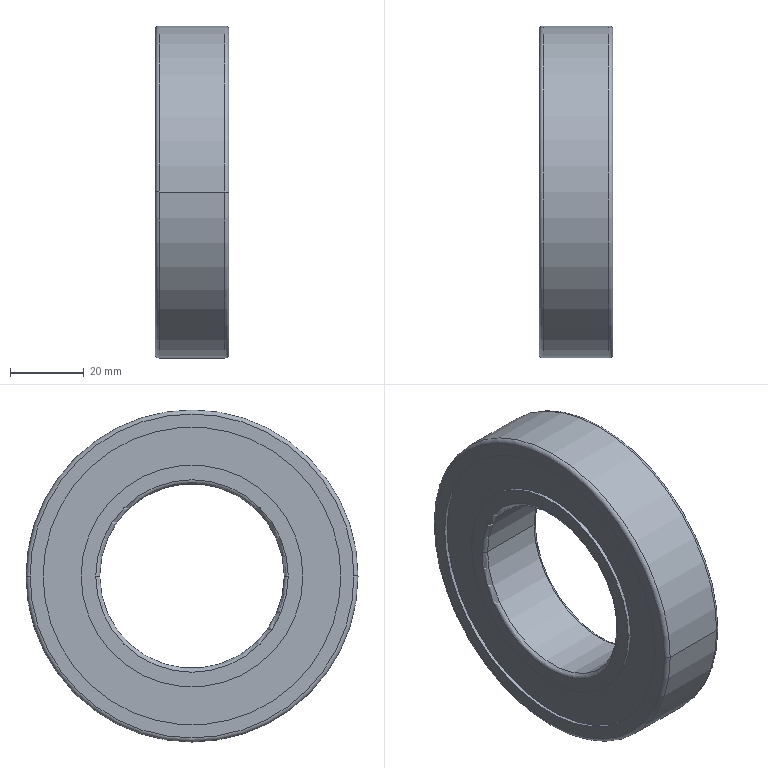Part | SolidWorks | features Fillet 2, Revolution 1 | 1 solid | 26 faces | box 20 x 90 x 90 mm | volume 83545 mm3 | cylinder 12 | torus 8 | plane 6 | commonest cylinder face diameters 60.1 x4 80.7 x4 50 x2 90 x2
STEP:
#1=CARTESIAN_POINT('',(1.1,-25.,0.));
#2=VERTEX_POINT('',#1);
#3=CARTESIAN_POINT('',(1.1,25.,0.));
#4=VERTEX_POINT('',#3);
#5=CARTESIAN_POINT('',(1.1,0.,0.));
#6=DIRECTION('',(-1.,0.,0.));
#7=DIRECTION('',(0.,1.,0.));
#8=AXIS2_PLACEMENT_3D('',#5,#6,#7);
#9=CIRCLE('',#8,25.);
#10=EDGE_CURVE('',#2,#4,#9,.T.);
#11=ORIENTED_EDGE('',*,*,#10,.F.);
#12=CARTESIAN_POINT('',(0.,-26.1,0.));
#13=VERTEX_POINT('',#12);
#14=CARTESIAN_POINT('',(1.1,-26.1,0.));
#15=DIRECTION('',(0.,0.,1.));
#16=DIRECTION('',(0.,-1.,0.));
#17=AXIS2_PLACEMENT_3D('',#14,#15,#16);
#18=CIRCLE('',#17,1.1);
#19=EDGE_CURVE('',#2,#13,#18,.T.);
#20=ORIENTED_EDGE('',*,*,#19,.T.);
#21=CARTESIAN_POINT('',(0.,26.1,0.));
#22=VERTEX_POINT('',#21);
#23=CARTESIAN_POINT('',(0.,0.,0.));
#24=DIRECTION('',(1.,0.,0.));
#25=DIRECTION('',(0.,1.,0.));
#26=AXIS2_PLACEMENT_3D('',#23,#24,#25);
#27=CIRCLE('',#26,26.1);
#28=EDGE_CURVE('',#22,#13,#27,.T.);
#29=ORIENTED_EDGE('',*,*,#28,.F.);
#30=CARTESIAN_POINT('',(1.1,26.1,0.));
#31=DIRECTION('',(0.,0.,-1.));
#32=DIRECTION('',(-1.,0.,0.));
#33=AXIS2_PLACEMENT_3D('',#30,#31,#32);
#34=CIRCLE('',#33,1.1);
#35=EDGE_CURVE('',#4,#22,#34,.T.);
#36=ORIENTED_EDGE('',*,*,#35,.F.);
#37=EDGE_LOOP('',(#11,#20,#29,#36));
#38=FACE_OUTER_BOUND('',#37,.T.);
#39=CARTESIAN_POINT('',(1.1,0.,0.));
#40=DIRECTION('',(1.,0.,0.));
#41=DIRECTION('',(0.,1.,0.));
#42=AXIS2_PLACEMENT_3D('',#39,#40,#41);
#43=TOROIDAL_SURFACE('',#42,26.1,1.1);
#44=ADVANCED_FACE('',(#38),#43,.T.);
#45=CARTESIAN_POINT('',(18.9,25.,0.));
#46=VERTEX_POINT('',#45);
#47=CARTESIAN_POINT('',(18.9,-25.,0.));
#48=VERTEX_POINT('',#47);
#49=CARTESIAN_POINT('',(18.9,0.,0.));
#50=DIRECTION('',(1.,0.,0.));
#51=DIRECTION('',(0.,-1.,0.));
#52=AXIS2_PLACEMENT_3D('',#49,#50,#51);
#53=CIRCLE('',#52,25.);
#54=EDGE_CURVE('',#46,#48,#53,.T.);
#55=ORIENTED_EDGE('',*,*,#54,.F.);
#56=CARTESIAN_POINT('',(20.,26.1,0.));
#57=VERTEX_POINT('',#56);
#58=CARTESIAN_POINT('',(18.9,26.1,0.));
#59=DIRECTION('',(0.,0.,1.));
#60=DIRECTION('',(0.,-1.,0.));
#61=AXIS2_PLACEMENT_3D('',#58,#59,#60);
#62=CIRCLE('',#61,1.1);
#63=EDGE_CURVE('',#46,#57,#62,.T.);
#64=ORIENTED_EDGE('',*,*,#63,.T.);
#65=CARTESIAN_POINT('',(20.,-26.1,0.));
#66=VERTEX_POINT('',#65);
#67=CARTESIAN_POINT('',(20.,0.,0.));
#68=DIRECTION('',(-1.,0.,0.));
#69=DIRECTION('',(0.,-1.,0.));
#70=AXIS2_PLACEMENT_3D('',#67,#68,#69);
#71=CIRCLE('',#70,26.1);
#72=EDGE_CURVE('',#66,#57,#71,.T.);
#73=ORIENTED_EDGE('',*,*,#72,.F.);
#74=CARTESIAN_POINT('',(18.9,-26.1,0.));
#75=DIRECTION('',(0.,0.,-1.));
#76=DIRECTION('',(-1.,0.,0.));
#77=AXIS2_PLACEMENT_3D('',#74,#75,#76);
#78=CIRCLE('',#77,1.1);
#79=EDGE_CURVE('',#48,#66,#78,.T.);
#80=ORIENTED_EDGE('',*,*,#79,.F.);
#81=EDGE_LOOP('',(#55,#64,#73,#80));
#82=FACE_OUTER_BOUND('',#81,.T.);
#83=CARTESIAN_POINT('',(18.9,0.,0.));
#84=DIRECTION('',(-1.,0.,0.));
#85=DIRECTION('',(0.,-1.,0.));
#86=AXIS2_PLACEMENT_3D('',#83,#84,#85);
#87=TOROIDAL_SURFACE('',#86,26.1,1.1);
#88=ADVANCED_FACE('',(#82),#87,.T.);
#89=CARTESIAN_POINT('',(0.,-43.9,0.));
#90=VERTEX_POINT('',#89);
#91=CARTESIAN_POINT('',(0.,43.9,0.));
#92=VERTEX_POINT('',#91);
#93=CARTESIAN_POINT('',(0.,0.,0.));
#94=DIRECTION('',(-1.,0.,0.));
#95=DIRECTION('',(0.,1.,0.));
#96=AXIS2_PLACEMENT_3D('',#93,#94,#95);
#97=CIRCLE('',#96,43.9);
#98=EDGE_CURVE('',#90,#92,#97,.T.);
#99=ORIENTED_EDGE('',*,*,#98,.F.);
#100=CARTESIAN_POINT('',(1.1,-45.,0.));
#101=VERTEX_POINT('',#100);
#102=CARTESIAN_POINT('',(1.1,-43.9,0.));
#103=DIRECTION('',(0.,0.,1.));
#104=DIRECTION('',(0.,-1.,0.));
#105=AXIS2_PLACEMENT_3D('',#102,#103,#104);
#106=CIRCLE('',#105,1.1);
#107=EDGE_CURVE('',#90,#101,#106,.T.);
#108=ORIENTED_EDGE('',*,*,#107,.T.);
#109=CARTESIAN_POINT('',(1.1,45.,0.));
#110=VERTEX_POINT('',#109);
#111=CARTESIAN_POINT('',(1.1,0.,0.));
#112=DIRECTION('',(1.,0.,0.));
#113=DIRECTION('',(0.,1.,0.));
#114=AXIS2_PLACEMENT_3D('',#111,#112,#113);
#115=CIRCLE('',#114,45.);
#116=EDGE_CURVE('',#110,#101,#115,.T.);
#117=ORIENTED_EDGE('',*,*,#116,.F.);
#118=CARTESIAN_POINT('',(1.1,43.9,0.));
#119=DIRECTION('',(0.,0.,-1.));
#120=DIRECTION('',(-1.,0.,0.));
#121=AXIS2_PLACEMENT_3D('',#118,#119,#120);
#122=CIRCLE('',#121,1.1);
#123=EDGE_CURVE('',#92,#110,#122,.T.);
#124=ORIENTED_EDGE('',*,*,#123,.F.);
#125=EDGE_LOOP('',(#99,#108,#117,#124));
#126=FACE_OUTER_BOUND('',#125,.T.);
#127=CARTESIAN_POINT('',(1.1,0.,0.));
#128=DIRECTION('',(1.,0.,0.));
#129=DIRECTION('',(0.,1.,0.));
#130=AXIS2_PLACEMENT_3D('',#127,#128,#129);
#131=TOROIDAL_SURFACE('',#130,43.9,1.1);
#132=ADVANCED_FACE('',(#126),#131,.T.);
#133=CARTESIAN_POINT('',(20.,43.9,0.));
#134=VERTEX_POINT('',#133);
#135=CARTESIAN_POINT('',(20.,-43.9,0.));
#136=VERTEX_POINT('',#135);
#137=CARTESIAN_POINT('',(20.,0.,0.));
#138=DIRECTION('',(1.,0.,0.));
#139=DIRECTION('',(0.,-1.,0.));
#140=AXIS2_PLACEMENT_3D('',#137,#138,#139);
#141=CIRCLE('',#140,43.9);
#142=EDGE_CURVE('',#134,#136,#141,.T.);
#143=ORIENTED_EDGE('',*,*,#142,.F.);
#144=CARTESIAN_POINT('',(18.9,45.,0.));
#145=VERTEX_POINT('',#144);
#146=CARTESIAN_POINT('',(18.9,43.9,0.));
#147=DIRECTION('',(0.,0.,1.));
#148=DIRECTION('',(0.,-1.,0.));
#149=AXIS2_PLACEMENT_3D('',#146,#147,#148);
#150=CIRCLE('',#149,1.1);
#151=EDGE_CURVE('',#134,#145,#150,.T.);
#152=ORIENTED_EDGE('',*,*,#151,.T.);
#153=CARTESIAN_POINT('',(18.9,-45.,0.));
#154=VERTEX_POINT('',#153);
#155=CARTESIAN_POINT('',(18.9,0.,0.));
#156=DIRECTION('',(-1.,0.,0.));
#157=DIRECTION('',(0.,-1.,0.));
#158=AXIS2_PLACEMENT_3D('',#155,#156,#157);
#159=CIRCLE('',#158,45.);
#160=EDGE_CURVE('',#154,#145,#159,.T.);
#161=ORIENTED_EDGE('',*,*,#160,.F.);
#162=CARTESIAN_POINT('',(18.9,-43.9,0.));
#163=DIRECTION('',(0.,0.,-1.));
#164=DIRECTION('',(-1.,0.,0.));
#165=AXIS2_PLACEMENT_3D('',#162,#163,#164);
#166=CIRCLE('',#165,1.1);
#167=EDGE_CURVE('',#136,#154,#166,.T.);
#168=ORIENTED_EDGE('',*,*,#167,.F.);
#169=EDGE_LOOP('',(#143,#152,#161,#168));
#170=FACE_OUTER_BOUND('',#169,.T.);
#171=CARTESIAN_POINT('',(18.9,0.,0.));
#172=DIRECTION('',(-1.,0.,0.));
#173=DIRECTION('',(0.,-1.,0.));
#174=AXIS2_PLACEMENT_3D('',#171,#172,#173);
#175=TOROIDAL_SURFACE('',#174,43.9,1.1);
#176=ADVANCED_FACE('',(#170),#175,.T.);
#177=ORIENTED_EDGE('',*,*,#160,.T.);
#178=CARTESIAN_POINT('',(0.,45.,0.));
#179=DIRECTION('',(-1.,0.,0.));
#180=VECTOR('',#179,1000.);
#181=LINE('',#178,#180);
#182=EDGE_CURVE('',#145,#110,#181,.T.);
#183=ORIENTED_EDGE('',*,*,#182,.T.);
#184=ORIENTED_EDGE('',*,*,#116,.T.);
#185=CARTESIAN_POINT('',(0.,-45.,0.));
#186=DIRECTION('',(-1.,0.,0.));
#187=VECTOR('',#186,1000.);
#188=LINE('',#185,#187);
#189=EDGE_CURVE('',#154,#101,#188,.T.);
#190=ORIENTED_EDGE('',*,*,#189,.F.);
#191=EDGE_LOOP('',(#177,#183,#184,#190));
#192=FACE_OUTER_BOUND('',#191,.T.);
#193=CARTESIAN_POINT('',(0.,0.,0.));
#194=DIRECTION('',(-1.,0.,0.));
#195=DIRECTION('',(0.,-1.,0.));
#196=AXIS2_PLACEMENT_3D('',#193,#194,#195);
#197=CYLINDRICAL_SURFACE('',#196,45.);
#198=ADVANCED_FACE('',(#192),#197,.T.);
#199=CARTESIAN_POINT('',(20.,40.35,0.));
#200=VERTEX_POINT('',#199);
#201=CARTESIAN_POINT('',(20.,-40.35,0.));
#202=VERTEX_POINT('',#201);
#203=CARTESIAN_POINT('',(20.,0.,0.));
#204=DIRECTION('',(-1.,0.,0.));
#205=DIRECTION('',(0.,-1.,0.));
#206=AXIS2_PLACEMENT_3D('',#203,#204,#205);
#207=CIRCLE('',#206,40.35);
#208=EDGE_CURVE('',#200,#202,#207,.T.);
#209=ORIENTED_EDGE('',*,*,#208,.F.);
#210=CARTESIAN_POINT('',(19.08,40.35,0.));
#211=VERTEX_POINT('',#210);
#212=CARTESIAN_POINT('',(0.,40.35,0.));
#213=DIRECTION('',(-1.,0.,0.));
#214=VECTOR('',#213,1000.);
#215=LINE('',#212,#214);
#216=EDGE_CURVE('',#200,#211,#215,.T.);
#217=ORIENTED_EDGE('',*,*,#216,.T.);
#218=CARTESIAN_POINT('',(19.08,-40.35,0.));
#219=VERTEX_POINT('',#218);
#220=CARTESIAN_POINT('',(19.08,0.,0.));
#221=DIRECTION('',(-1.,0.,0.));
#222=DIRECTION('',(0.,-1.,0.));
#223=AXIS2_PLACEMENT_3D('',#220,#221,#222);
#224=CIRCLE('',#223,40.35);
#225=EDGE_CURVE('',#211,#219,#224,.T.);
#226=ORIENTED_EDGE('',*,*,#225,.T.);
#227=CARTESIAN_POINT('',(0.,-40.35,0.));
#228=DIRECTION('',(-1.,0.,0.));
#229=VECTOR('',#228,1000.);
#230=LINE('',#227,#229);
#231=EDGE_CURVE('',#202,#219,#230,.T.);
#232=ORIENTED_EDGE('',*,*,#231,.F.);
#233=EDGE_LOOP('',(#209,#217,#226,#232));
#234=FACE_OUTER_BOUND('',#233,.T.);
#235=CARTESIAN_POINT('',(0.,0.,0.));
#236=DIRECTION('',(-1.,0.,0.));
#237=DIRECTION('',(0.,-1.,0.));
#238=AXIS2_PLACEMENT_3D('',#235,#236,#237);
#239=CYLINDRICAL_SURFACE('',#238,40.35);
#240=ADVANCED_FACE('',(#234),#239,.F.);
#241=CARTESIAN_POINT('',(20.,-30.05,0.));
#242=VERTEX_POINT('',#241);
#243=CARTESIAN_POINT('',(20.,30.05,0.));
#244=VERTEX_POINT('',#243);
#245=CARTESIAN_POINT('',(20.,0.,0.));
#246=DIRECTION('',(-1.,0.,0.));
#247=DIRECTION('',(0.,-1.,0.));
#248=AXIS2_PLACEMENT_3D('',#245,#246,#247);
#249=CIRCLE('',#248,30.05);
#250=EDGE_CURVE('',#242,#244,#249,.T.);
#251=ORIENTED_EDGE('',*,*,#250,.T.);
#252=CARTESIAN_POINT('',(19.08,30.05,0.));
#253=VERTEX_POINT('',#252);
#254=CARTESIAN_POINT('',(0.,30.05,0.));
#255=DIRECTION('',(-1.,0.,0.));
#256=VECTOR('',#255,1000.);
#257=LINE('',#254,#256);
#258=EDGE_CURVE('',#244,#253,#257,.T.);
#259=ORIENTED_EDGE('',*,*,#258,.T.);
#260=CARTESIAN_POINT('',(19.08,-30.05,0.));
#261=VERTEX_POINT('',#260);
#262=CARTESIAN_POINT('',(19.08,0.,0.));
#263=DIRECTION('',(-1.,0.,0.));
#264=DIRECTION('',(0.,-1.,0.));
#265=AXIS2_PLACEMENT_3D('',#262,#263,#264);
#266=CIRCLE('',#265,30.05);
#267=EDGE_CURVE('',#261,#253,#266,.T.);
#268=ORIENTED_EDGE('',*,*,#267,.F.);
#269=CARTESIAN_POINT('',(0.,-30.05,0.));
#270=DIRECTION('',(-1.,0.,0.));
#271=VECTOR('',#270,1000.);
#272=LINE('',#269,#271);
#273=EDGE_CURVE('',#242,#261,#272,.T.);
#274=ORIENTED_EDGE('',*,*,#273,.F.);
#275=EDGE_LOOP('',(#251,#259,#268,#274));
#276=FACE_OUTER_BOUND('',#275,.T.);
#277=CARTESIAN_POINT('',(0.,0.,0.));
#278=DIRECTION('',(-1.,0.,0.));
#279=DIRECTION('',(0.,-1.,0.));
#280=AXIS2_PLACEMENT_3D('',#277,#278,#279);
#281=CYLINDRICAL_SURFACE('',#280,30.05);
#282=ADVANCED_FACE('',(#276),#281,.T.);
#283=CARTESIAN_POINT('',(18.9,0.,0.));
#284=DIRECTION('',(1.,0.,0.));
#285=DIRECTION('',(0.,-1.,0.));
#286=AXIS2_PLACEMENT_3D('',#283,#284,#285);
#287=CIRCLE('',#286,25.);
#288=EDGE_CURVE('',#48,#46,#287,.T.);
#289=ORIENTED_EDGE('',*,*,#288,.T.);
#290=CARTESIAN_POINT('',(0.,25.,0.));
#291=DIRECTION('',(-1.,0.,0.));
#292=VECTOR('',#291,1000.);
#293=LINE('',#290,#292);
#294=EDGE_CURVE('',#46,#4,#293,.T.);
#295=ORIENTED_EDGE('',*,*,#294,.T.);
#296=CARTESIAN_POINT('',(1.1,0.,0.));
#297=DIRECTION('',(-1.,0.,0.));
#298=DIRECTION('',(0.,1.,0.));
#299=AXIS2_PLACEMENT_3D('',#296,#297,#298);
#300=CIRCLE('',#299,25.);
#301=EDGE_CURVE('',#4,#2,#300,.T.);
#302=ORIENTED_EDGE('',*,*,#301,.T.);
#303=CARTESIAN_POINT('',(0.,-25.,0.));
#304=DIRECTION('',(-1.,0.,0.));
#305=VECTOR('',#304,1000.);
#306=LINE('',#303,#305);
#307=EDGE_CURVE('',#48,#2,#306,.T.);
#308=ORIENTED_EDGE('',*,*,#307,.F.);
#309=EDGE_LOOP('',(#289,#295,#302,#308));
#310=FACE_OUTER_BOUND('',#309,.T.);
#311=CARTESIAN_POINT('',(0.,0.,0.));
#312=DIRECTION('',(-1.,0.,0.));
#313=DIRECTION('',(0.,-1.,0.));
#314=AXIS2_PLACEMENT_3D('',#311,#312,#313);
#315=CYLINDRICAL_SURFACE('',#314,25.);
#316=ADVANCED_FACE('',(#310),#315,.F.);
#317=CARTESIAN_POINT('',(0.92,-30.05,0.));
#318=VERTEX_POINT('',#317);
#319=CARTESIAN_POINT('',(0.92,30.05,0.));
#320=VERTEX_POINT('',#319);
#321=CARTESIAN_POINT('',(0.92,0.,0.));
#322=DIRECTION('',(-1.,0.,0.));
#323=DIRECTION('',(0.,-1.,0.));
#324=AXIS2_PLACEMENT_3D('',#321,#322,#323);
#325=CIRCLE('',#324,30.05);
#326=EDGE_CURVE('',#318,#320,#325,.T.);
#327=ORIENTED_EDGE('',*,*,#326,.T.);
#328=CARTESIAN_POINT('',(0.,30.05,0.));
#329=VERTEX_POINT('',#328);
#330=CARTESIAN_POINT('',(0.,30.05,0.));
#331=DIRECTION('',(-1.,0.,0.));
#332=VECTOR('',#331,1000.);
#333=LINE('',#330,#332);
#334=EDGE_CURVE('',#320,#329,#333,.T.);
#335=ORIENTED_EDGE('',*,*,#334,.T.);
#336=CARTESIAN_POINT('',(0.,-30.05,0.));
#337=VERTEX_POINT('',#336);
#338=CARTESIAN_POINT('',(0.,0.,0.));
#339=DIRECTION('',(-1.,0.,0.));
#340=DIRECTION('',(0.,-1.,0.));
#341=AXIS2_PLACEMENT_3D('',#338,#339,#340);
#342=CIRCLE('',#341,30.05);
#343=EDGE_CURVE('',#337,#329,#342,.T.);
#344=ORIENTED_EDGE('',*,*,#343,.F.);
#345=CARTESIAN_POINT('',(0.,-30.05,0.));
#346=DIRECTION('',(-1.,0.,0.));
#347=VECTOR('',#346,1000.);
#348=LINE('',#345,#347);
#349=EDGE_CURVE('',#318,#337,#348,.T.);
#350=ORIENTED_EDGE('',*,*,#349,.F.);
#351=EDGE_LOOP('',(#327,#335,#344,#350));
#352=FACE_OUTER_BOUND('',#351,.T.);
#353=CARTESIAN_POINT('',(0.,0.,0.));
#354=DIRECTION('',(-1.,0.,0.));
#355=DIRECTION('',(0.,-1.,0.));
#356=AXIS2_PLACEMENT_3D('',#353,#354,#355);
#357=CYLINDRICAL_SURFACE('',#356,30.05);
#358=ADVANCED_FACE('',(#352),#357,.T.);
#359=CARTESIAN_POINT('',(0.92,40.35,0.));
#360=VERTEX_POINT('',#359);
#361=CARTESIAN_POINT('',(0.92,-40.35,0.));
#362=VERTEX_POINT('',#361);
#363=CARTESIAN_POINT('',(0.92,0.,0.));
#364=DIRECTION('',(-1.,0.,0.));
#365=DIRECTION('',(0.,-1.,0.));
#366=AXIS2_PLACEMENT_3D('',#363,#364,#365);
#367=CIRCLE('',#366,40.35);
#368=EDGE_CURVE('',#360,#362,#367,.T.);
#369=ORIENTED_EDGE('',*,*,#368,.F.);
#370=CARTESIAN_POINT('',(0.,40.35,0.));
#371=VERTEX_POINT('',#370);
#372=CARTESIAN_POINT('',(0.,40.35,0.));
#373=DIRECTION('',(-1.,0.,0.));
#374=VECTOR('',#373,1000.);
#375=LINE('',#372,#374);
#376=EDGE_CURVE('',#360,#371,#375,.T.);
#377=ORIENTED_EDGE('',*,*,#376,.T.);
#378=CARTESIAN_POINT('',(0.,-40.35,0.));
#379=VERTEX_POINT('',#378);
#380=CARTESIAN_POINT('',(0.,0.,0.));
#381=DIRECTION('',(-1.,0.,0.));
#382=DIRECTION('',(0.,-1.,0.));
#383=AXIS2_PLACEMENT_3D('',#380,#381,#382);
#384=CIRCLE('',#383,40.35);
#385=EDGE_CURVE('',#371,#379,#384,.T.);
#386=ORIENTED_EDGE('',*,*,#385,.T.);
#387=CARTESIAN_POINT('',(0.,-40.35,0.));
#388=DIRECTION('',(-1.,0.,0.));
#389=VECTOR('',#388,1000.);
#390=LINE('',#387,#389);
#391=EDGE_CURVE('',#362,#379,#390,.T.);
#392=ORIENTED_EDGE('',*,*,#391,.F.);
#393=EDGE_LOOP('',(#369,#377,#386,#392));
#394=FACE_OUTER_BOUND('',#393,.T.);
#395=CARTESIAN_POINT('',(0.,0.,0.));
#396=DIRECTION('',(-1.,0.,0.));
#397=DIRECTION('',(0.,-1.,0.));
#398=AXIS2_PLACEMENT_3D('',#395,#396,#397);
#399=CYLINDRICAL_SURFACE('',#398,40.35);
#400=ADVANCED_FACE('',(#394),#399,.F.);
#401=CARTESIAN_POINT('',(0.,0.,0.));
#402=DIRECTION('',(-1.,0.,0.));
#403=DIRECTION('',(0.,1.,0.));
#404=AXIS2_PLACEMENT_3D('',#401,#402,#403);
#405=CIRCLE('',#404,43.9);
#406=EDGE_CURVE('',#92,#90,#405,.T.);
#407=ORIENTED_EDGE('',*,*,#406,.T.);
#408=ORIENTED_EDGE('',*,*,#98,.T.);
#409=EDGE_LOOP('',(#407,#408));
#410=FACE_OUTER_BOUND('',#409,.T.);
#411=CARTESIAN_POINT('',(0.,0.,0.));
#412=DIRECTION('',(-1.,0.,0.));
#413=DIRECTION('',(0.,-1.,0.));
#414=AXIS2_PLACEMENT_3D('',#411,#412,#413);
#415=CIRCLE('',#414,40.35);
#416=EDGE_CURVE('',#379,#371,#415,.T.);
#417=ORIENTED_EDGE('',*,*,#416,.F.);
#418=ORIENTED_EDGE('',*,*,#385,.F.);
#419=EDGE_LOOP('',(#417,#418));
#420=FACE_BOUND('',#419,.T.);
#421=CARTESIAN_POINT('',(0.,45.,0.));
#422=DIRECTION('',(1.,0.,0.));
#423=DIRECTION('',(0.,1.,0.));
#424=AXIS2_PLACEMENT_3D('',#421,#422,#423);
#425=PLANE('',#424);
#426=ADVANCED_FACE('',(#410,#420),#425,.F.);
#427=ORIENTED_EDGE('',*,*,#376,.F.);
#428=CARTESIAN_POINT('',(0.92,0.,0.));
#429=DIRECTION('',(-1.,0.,0.));
#430=DIRECTION('',(0.,-1.,0.));
#431=AXIS2_PLACEMENT_3D('',#428,#429,#430);
#432=CIRCLE('',#431,40.35);
#433=EDGE_CURVE('',#362,#360,#432,.T.);
#434=ORIENTED_EDGE('',*,*,#433,.F.);
#435=ORIENTED_EDGE('',*,*,#391,.T.);
#436=ORIENTED_EDGE('',*,*,#416,.T.);
#437=EDGE_LOOP('',(#427,#434,#435,#436));
#438=FACE_OUTER_BOUND('',#437,.T.);
#439=CARTESIAN_POINT('',(0.,0.,0.));
#440=DIRECTION('',(-1.,0.,0.));
#441=DIRECTION('',(0.,-1.,0.));
#442=AXIS2_PLACEMENT_3D('',#439,#440,#441);
#443=CYLINDRICAL_SURFACE('',#442,40.35);
#444=ADVANCED_FACE('',(#438),#443,.F.);
#445=ORIENTED_EDGE('',*,*,#326,.F.);
#446=CARTESIAN_POINT('',(0.92,0.,0.));
#447=DIRECTION('',(-1.,0.,0.));
#448=DIRECTION('',(0.,-1.,0.));
#449=AXIS2_PLACEMENT_3D('',#446,#447,#448);
#450=CIRCLE('',#449,30.05);
#451=EDGE_CURVE('',#320,#318,#450,.T.);
#452=ORIENTED_EDGE('',*,*,#451,.F.);
#453=EDGE_LOOP('',(#445,#452));
#454=FACE_BOUND('',#453,.T.);
#455=ORIENTED_EDGE('',*,*,#433,.T.);
#456=ORIENTED_EDGE('',*,*,#368,.T.);
#457=EDGE_LOOP('',(#455,#456));
#458=FACE_OUTER_BOUND('',#457,.T.);
#459=CARTESIAN_POINT('',(0.92,40.35,0.));
#460=DIRECTION('',(1.,0.,0.));
#461=DIRECTION('',(0.,1.,0.));
#462=AXIS2_PLACEMENT_3D('',#459,#460,#461);
#463=PLANE('',#462);
#464=ADVANCED_FACE('',(#454,#458),#463,.F.);
#465=ORIENTED_EDGE('',*,*,#334,.F.);
#466=ORIENTED_EDGE('',*,*,#451,.T.);
#467=ORIENTED_EDGE('',*,*,#349,.T.);
#468=CARTESIAN_POINT('',(0.,0.,0.));
#469=DIRECTION('',(-1.,0.,0.));
#470=DIRECTION('',(0.,-1.,0.));
#471=AXIS2_PLACEMENT_3D('',#468,#469,#470);
#472=CIRCLE('',#471,30.05);
#473=EDGE_CURVE('',#329,#337,#472,.T.);
#474=ORIENTED_EDGE('',*,*,#473,.F.);
#475=EDGE_LOOP('',(#465,#466,#467,#474));
#476=FACE_OUTER_BOUND('',#475,.T.);
#477=CARTESIAN_POINT('',(0.,0.,0.));
#478=DIRECTION('',(-1.,0.,0.));
#479=DIRECTION('',(0.,-1.,0.));
#480=AXIS2_PLACEMENT_3D('',#477,#478,#479);
#481=CYLINDRICAL_SURFACE('',#480,30.05);
#482=ADVANCED_FACE('',(#476),#481,.T.);
#483=ORIENTED_EDGE('',*,*,#28,.T.);
#484=CARTESIAN_POINT('',(0.,0.,0.));
#485=DIRECTION('',(1.,0.,0.));
#486=DIRECTION('',(0.,1.,0.));
#487=AXIS2_PLACEMENT_3D('',#484,#485,#486);
#488=CIRCLE('',#487,26.1);
#489=EDGE_CURVE('',#13,#22,#488,.T.);
#490=ORIENTED_EDGE('',*,*,#489,.T.);
#491=EDGE_LOOP('',(#483,#490));
#492=FACE_BOUND('',#491,.T.);
#493=ORIENTED_EDGE('',*,*,#343,.T.);
#494=ORIENTED_EDGE('',*,*,#473,.T.);
#495=EDGE_LOOP('',(#493,#494));
#496=FACE_OUTER_BOUND('',#495,.T.);
#497=CARTESIAN_POINT('',(0.,30.05,0.));
#498=DIRECTION('',(1.,0.,0.));
#499=DIRECTION('',(0.,1.,0.));
#500=AXIS2_PLACEMENT_3D('',#497,#498,#499);
#501=PLANE('',#500);
#502=ADVANCED_FACE('',(#492,#496),#501,.F.);
#503=ORIENTED_EDGE('',*,*,#294,.F.);
#504=ORIENTED_EDGE('',*,*,#54,.T.);
#505=ORIENTED_EDGE('',*,*,#307,.T.);
#506=ORIENTED_EDGE('',*,*,#10,.T.);
#507=EDGE_LOOP('',(#503,#504,#505,#506));
#508=FACE_OUTER_BOUND('',#507,.T.);
#509=CARTESIAN_POINT('',(0.,0.,0.));
#510=DIRECTION('',(-1.,0.,0.));
#511=DIRECTION('',(0.,-1.,0.));
#512=AXIS2_PLACEMENT_3D('',#509,#510,#511);
#513=CYLINDRICAL_SURFACE('',#512,25.);
#514=ADVANCED_FACE('',(#508),#513,.F.);
#515=ORIENTED_EDGE('',*,*,#72,.T.);
#516=CARTESIAN_POINT('',(20.,0.,0.));
#517=DIRECTION('',(-1.,0.,0.));
#518=DIRECTION('',(0.,-1.,0.));
#519=AXIS2_PLACEMENT_3D('',#516,#517,#518);
#520=CIRCLE('',#519,26.1);
#521=EDGE_CURVE('',#57,#66,#520,.T.);
#522=ORIENTED_EDGE('',*,*,#521,.T.);
#523=EDGE_LOOP('',(#515,#522));
#524=FACE_BOUND('',#523,.T.);
#525=ORIENTED_EDGE('',*,*,#250,.F.);
#526=CARTESIAN_POINT('',(20.,0.,0.));
#527=DIRECTION('',(-1.,0.,0.));
#528=DIRECTION('',(0.,-1.,0.));
#529=AXIS2_PLACEMENT_3D('',#526,#527,#528);
#530=CIRCLE('',#529,30.05);
#531=EDGE_CURVE('',#244,#242,#530,.T.);
#532=ORIENTED_EDGE('',*,*,#531,.F.);
#533=EDGE_LOOP('',(#525,#532));
#534=FACE_OUTER_BOUND('',#533,.T.);
#535=CARTESIAN_POINT('',(20.,30.05,0.));
#536=DIRECTION('',(-1.,0.,0.));
#537=DIRECTION('',(0.,-1.,0.));
#538=AXIS2_PLACEMENT_3D('',#535,#536,#537);
#539=PLANE('',#538);
#540=ADVANCED_FACE('',(#524,#534),#539,.F.);
#541=ORIENTED_EDGE('',*,*,#258,.F.);
#542=ORIENTED_EDGE('',*,*,#531,.T.);
#543=ORIENTED_EDGE('',*,*,#273,.T.);
#544=CARTESIAN_POINT('',(19.08,0.,0.));
#545=DIRECTION('',(-1.,0.,0.));
#546=DIRECTION('',(0.,-1.,0.));
#547=AXIS2_PLACEMENT_3D('',#544,#545,#546);
#548=CIRCLE('',#547,30.05);
#549=EDGE_CURVE('',#253,#261,#548,.T.);
#550=ORIENTED_EDGE('',*,*,#549,.F.);
#551=EDGE_LOOP('',(#541,#542,#543,#550));
#552=FACE_OUTER_BOUND('',#551,.T.);
#553=CARTESIAN_POINT('',(0.,0.,0.));
#554=DIRECTION('',(-1.,0.,0.));
#555=DIRECTION('',(0.,-1.,0.));
#556=AXIS2_PLACEMENT_3D('',#553,#554,#555);
#557=CYLINDRICAL_SURFACE('',#556,30.05);
#558=ADVANCED_FACE('',(#552),#557,.T.);
#559=CARTESIAN_POINT('',(19.08,0.,0.));
#560=DIRECTION('',(-1.,0.,0.));
#561=DIRECTION('',(0.,-1.,0.));
#562=AXIS2_PLACEMENT_3D('',#559,#560,#561);
#563=CIRCLE('',#562,40.35);
#564=EDGE_CURVE('',#219,#211,#563,.T.);
#565=ORIENTED_EDGE('',*,*,#564,.F.);
#566=ORIENTED_EDGE('',*,*,#225,.F.);
#567=EDGE_LOOP('',(#565,#566));
#568=FACE_OUTER_BOUND('',#567,.T.);
#569=ORIENTED_EDGE('',*,*,#267,.T.);
#570=ORIENTED_EDGE('',*,*,#549,.T.);
#571=EDGE_LOOP('',(#569,#570));
#572=FACE_BOUND('',#571,.T.);
#573=CARTESIAN_POINT('',(19.08,40.35,0.));
#574=DIRECTION('',(-1.,0.,0.));
#575=DIRECTION('',(0.,-1.,0.));
#576=AXIS2_PLACEMENT_3D('',#573,#574,#575);
#577=PLANE('',#576);
#578=ADVANCED_FACE('',(#568,#572),#577,.F.);
#579=ORIENTED_EDGE('',*,*,#216,.F.);
#580=CARTESIAN_POINT('',(20.,0.,0.));
#581=DIRECTION('',(-1.,0.,0.));
#582=DIRECTION('',(0.,-1.,0.));
#583=AXIS2_PLACEMENT_3D('',#580,#581,#582);
#584=CIRCLE('',#583,40.35);
#585=EDGE_CURVE('',#202,#200,#584,.T.);
#586=ORIENTED_EDGE('',*,*,#585,.F.);
#587=ORIENTED_EDGE('',*,*,#231,.T.);
#588=ORIENTED_EDGE('',*,*,#564,.T.);
#589=EDGE_LOOP('',(#579,#586,#587,#588));
#590=FACE_OUTER_BOUND('',#589,.T.);
#591=CARTESIAN_POINT('',(0.,0.,0.));
#592=DIRECTION('',(-1.,0.,0.));
#593=DIRECTION('',(0.,-1.,0.));
#594=AXIS2_PLACEMENT_3D('',#591,#592,#593);
#595=CYLINDRICAL_SURFACE('',#594,40.35);
#596=ADVANCED_FACE('',(#590),#595,.F.);
#597=CARTESIAN_POINT('',(20.,0.,0.));
#598=DIRECTION('',(1.,0.,0.));
#599=DIRECTION('',(0.,-1.,0.));
#600=AXIS2_PLACEMENT_3D('',#597,#598,#599);
#601=CIRCLE('',#600,43.9);
#602=EDGE_CURVE('',#136,#134,#601,.T.);
#603=ORIENTED_EDGE('',*,*,#602,.T.);
#604=ORIENTED_EDGE('',*,*,#142,.T.);
#605=EDGE_LOOP('',(#603,#604));
#606=FACE_OUTER_BOUND('',#605,.T.);
#607=ORIENTED_EDGE('',*,*,#585,.T.);
#608=ORIENTED_EDGE('',*,*,#208,.T.);
#609=EDGE_LOOP('',(#607,#608));
#610=FACE_BOUND('',#609,.T.);
#611=CARTESIAN_POINT('',(20.,45.,0.));
#612=DIRECTION('',(-1.,0.,0.));
#613=DIRECTION('',(0.,-1.,0.));
#614=AXIS2_PLACEMENT_3D('',#611,#612,#613);
#615=PLANE('',#614);
#616=ADVANCED_FACE('',(#606,#610),#615,.F.);
#617=ORIENTED_EDGE('',*,*,#182,.F.);
#618=CARTESIAN_POINT('',(18.9,0.,0.));
#619=DIRECTION('',(-1.,0.,0.));
#620=DIRECTION('',(0.,-1.,0.));
#621=AXIS2_PLACEMENT_3D('',#618,#619,#620);
#622=CIRCLE('',#621,45.);
#623=EDGE_CURVE('',#145,#154,#622,.T.);
#624=ORIENTED_EDGE('',*,*,#623,.T.);
#625=ORIENTED_EDGE('',*,*,#189,.T.);
#626=CARTESIAN_POINT('',(1.1,0.,0.));
#627=DIRECTION('',(1.,0.,0.));
#628=DIRECTION('',(0.,1.,0.));
#629=AXIS2_PLACEMENT_3D('',#626,#627,#628);
#630=CIRCLE('',#629,45.);
#631=EDGE_CURVE('',#101,#110,#630,.T.);
#632=ORIENTED_EDGE('',*,*,#631,.T.);
#633=EDGE_LOOP('',(#617,#624,#625,#632));
#634=FACE_OUTER_BOUND('',#633,.T.);
#635=CARTESIAN_POINT('',(0.,0.,0.));
#636=DIRECTION('',(-1.,0.,0.));
#637=DIRECTION('',(0.,-1.,0.));
#638=AXIS2_PLACEMENT_3D('',#635,#636,#637);
#639=CYLINDRICAL_SURFACE('',#638,45.);
#640=ADVANCED_FACE('',(#634),#639,.T.);
#641=ORIENTED_EDGE('',*,*,#151,.F.);
#642=ORIENTED_EDGE('',*,*,#602,.F.);
#643=ORIENTED_EDGE('',*,*,#167,.T.);
#644=ORIENTED_EDGE('',*,*,#623,.F.);
#645=EDGE_LOOP('',(#641,#642,#643,#644));
#646=FACE_OUTER_BOUND('',#645,.T.);
#647=CARTESIAN_POINT('',(18.9,0.,0.));
#648=DIRECTION('',(-1.,0.,0.));
#649=DIRECTION('',(0.,-1.,0.));
#650=AXIS2_PLACEMENT_3D('',#647,#648,#649);
#651=TOROIDAL_SURFACE('',#650,43.9,1.1);
#652=ADVANCED_FACE('',(#646),#651,.T.);
#653=ORIENTED_EDGE('',*,*,#107,.F.);
#654=ORIENTED_EDGE('',*,*,#406,.F.);
#655=ORIENTED_EDGE('',*,*,#123,.T.);
#656=ORIENTED_EDGE('',*,*,#631,.F.);
#657=EDGE_LOOP('',(#653,#654,#655,#656));
#658=FACE_OUTER_BOUND('',#657,.T.);
#659=CARTESIAN_POINT('',(1.1,0.,0.));
#660=DIRECTION('',(1.,0.,0.));
#661=DIRECTION('',(0.,1.,0.));
#662=AXIS2_PLACEMENT_3D('',#659,#660,#661);
#663=TOROIDAL_SURFACE('',#662,43.9,1.1);
#664=ADVANCED_FACE('',(#658),#663,.T.);
#665=ORIENTED_EDGE('',*,*,#63,.F.);
#666=ORIENTED_EDGE('',*,*,#288,.F.);
#667=ORIENTED_EDGE('',*,*,#79,.T.);
#668=ORIENTED_EDGE('',*,*,#521,.F.);
#669=EDGE_LOOP('',(#665,#666,#667,#668));
#670=FACE_OUTER_BOUND('',#669,.T.);
#671=CARTESIAN_POINT('',(18.9,0.,0.));
#672=DIRECTION('',(-1.,0.,0.));
#673=DIRECTION('',(0.,-1.,0.));
#674=AXIS2_PLACEMENT_3D('',#671,#672,#673);
#675=TOROIDAL_SURFACE('',#674,26.1,1.1);
#676=ADVANCED_FACE('',(#670),#675,.T.);
#677=ORIENTED_EDGE('',*,*,#19,.F.);
#678=ORIENTED_EDGE('',*,*,#301,.F.);
#679=ORIENTED_EDGE('',*,*,#35,.T.);
#680=ORIENTED_EDGE('',*,*,#489,.F.);
#681=EDGE_LOOP('',(#677,#678,#679,#680));
#682=FACE_OUTER_BOUND('',#681,.T.);
#683=CARTESIAN_POINT('',(1.1,0.,0.));
#684=DIRECTION('',(1.,0.,0.));
#685=DIRECTION('',(0.,1.,0.));
#686=AXIS2_PLACEMENT_3D('',#683,#684,#685);
#687=TOROIDAL_SURFACE('',#686,26.1,1.1);
#688=ADVANCED_FACE('',(#682),#687,.T.);
#689=CLOSED_SHELL('',(#44,#88,#132,#176,#198,#240,#282,#316,#358,#400,#426,#444,#464,#482,#502,#514,#540,#558,#578,#596,#616,#640,#652,#664,#676,#688));
#690=MANIFOLD_SOLID_BREP('',#689);
#691=CARTESIAN_POINT('',(0.,0.,0.));
#692=DIRECTION('',(0.,0.,1.));
#693=DIRECTION('',(1.,0.,0.));
#694=AXIS2_PLACEMENT_3D('',#691,#692,#693);
#695=(LENGTH_UNIT()NAMED_UNIT(*)SI_UNIT(.MILLI.,.METRE.));
#696=UNCERTAINTY_MEASURE_WITH_UNIT(LENGTH_MEASURE(0.00001),#695,'','');
#697=(NAMED_UNIT(*)PLANE_ANGLE_UNIT()SI_UNIT($,.RADIAN.));
#698=(NAMED_UNIT(*)SI_UNIT($,.STERADIAN.)SOLID_ANGLE_UNIT());
#699=(GEOMETRIC_REPRESENTATION_CONTEXT(3)GLOBAL_UNCERTAINTY_ASSIGNED_CONTEXT((#696))GLOBAL_UNIT_ASSIGNED_CONTEXT((#695,#697,#698))REPRESENTATION_CONTEXT('',''));
#700=ADVANCED_BREP_SHAPE_REPRESENTATION('',(#690,#694),#699);